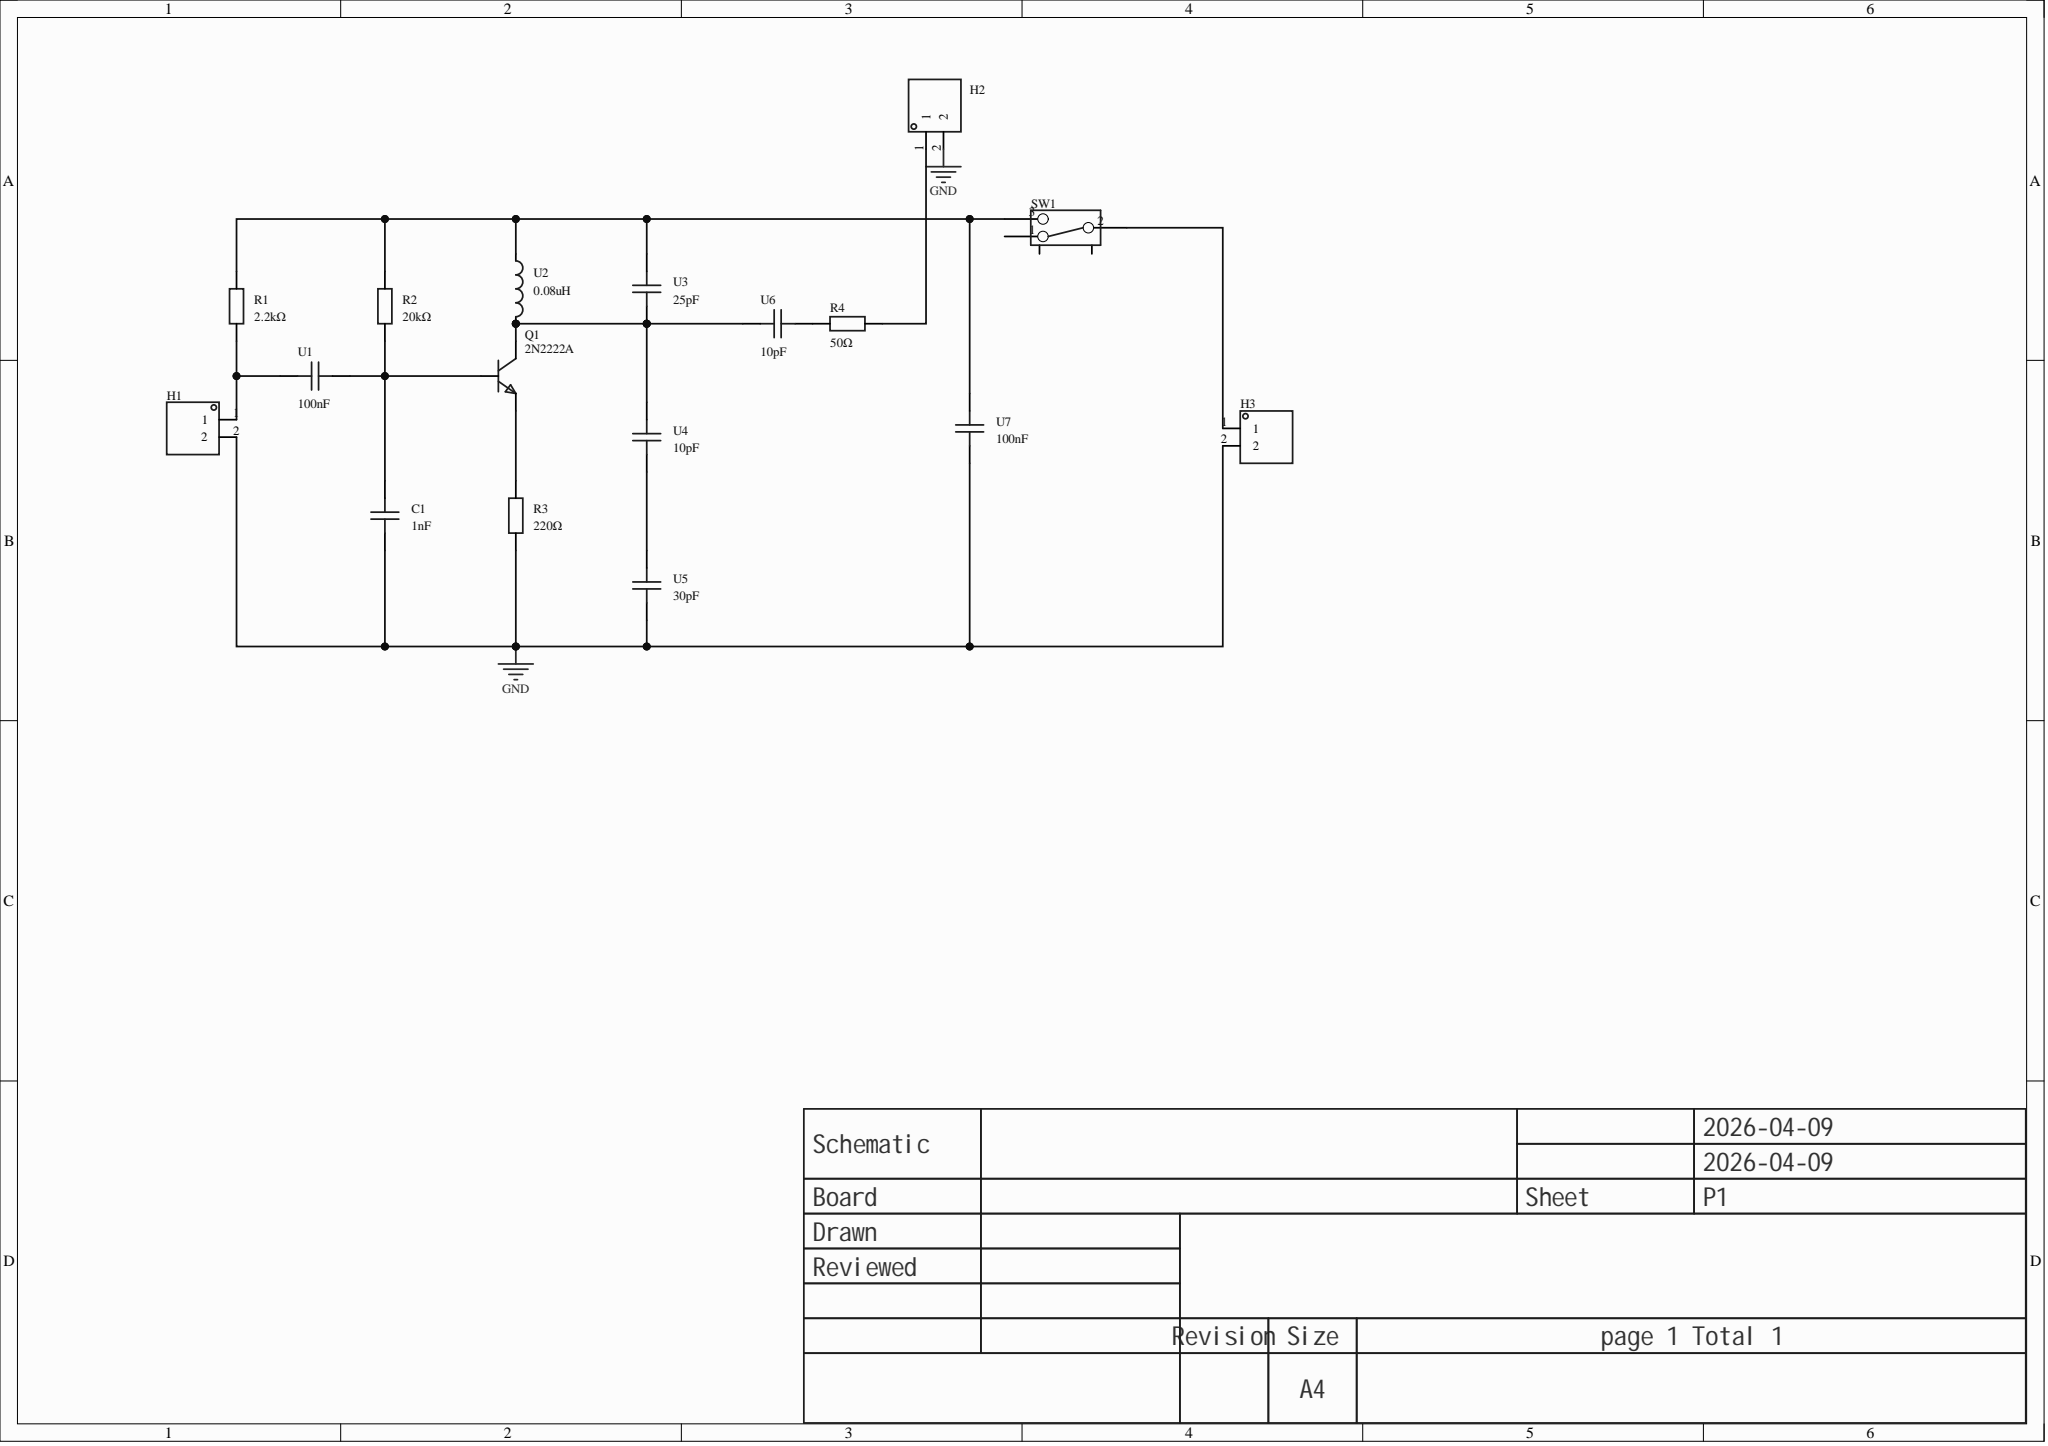Circuit board | Altium Designer | 17 parts | 10 nets
Bill of materials:
Comment,Description,Designator,Footprint,LibRef,Quantity
"1nF","Capacitance: 1nF; Tolerance: ±20%; Working voltage (AC): 400V; 440V; Protection class: X1,Y1;","C1","CAP-TH_L7.0-W4.0-P10.00-D0.6-1","DE1E3RA102MJ4BH01F","1"
"","","H1, H2, H3","HDR-TH_2P-P2.54-V-M-1","HDR-M_2.54_1x2P","3"
"2N2222A","Transistor type: NPN.  Collector current ICM: 800MA  Collector-base breakdown voltage BVCBO: 60V  Collector-emitter breakdown voltage BVCEO: 30V  DC current gain HFE: 100-200","Q1","TO-92-3_L5.1-W4.1-P1.27-L-1","2N2222A_C50229645","1"
"2.2kΩ","","R1","Res_1/8W","Res_AXIAL-1/8W","1"
"20kΩ","","R2","Res_1/8W","Res_AXIAL-1/8W","1"
"220Ω","","R3","Res_1/8W","Res_AXIAL-1/8W","1"
"50Ω","","R4","Res_1/8W","Res_AXIAL-1/8W","1"
"","","SW1","拨动开关_侧","拨动开关_侧","1"
"100nF","","U1, U7","CAP-TH_L5.0-W2.5-P5.00-D1.0","100nF","2"
"0.08uH","Inductance: 1uH; Tolerance: ±10%; Rated current: 4.45A; Saturation current (Isat): 7.7A; Type: color-band inductor; Quality factor: 50@2.52MHz;","U2","IND-TH_BD6.5-W9.2-LS14.0-D0.8","B82144F2102K000","1"
"25pF","","U3","CAP-TH_L5.0-W2.5-P5.00-D1.0","100nF","1"
"10pF","","U4, U6","CAP-TH_L5.0-W2.5-P5.00-D1.0","100nF","2"
"30pF","","U5","CAP-TH_L5.0-W2.5-P5.00-D1.0","100nF","1"
Netlist (Protel format):
[
C1
CAP-TH_L7.0-W4.0-P10.00-D0.6-1
1nF



]
[
H1
HDR-TH_2P-P2.54-V-M-1




]
[
H2
HDR-TH_2P-P2.54-V-M-1




]
[
H3
HDR-TH_2P-P2.54-V-M-1




]
[
Q1
TO-92-3_L5.1-W4.1-P1.27-L-1
2N2222A



]
[
R1
Res_1/8W
2.2kΩ



]
[
R2
Res_1/8W
20kΩ



]
[
R3
Res_1/8W
220Ω



]
[
R4
Res_1/8W
50Ω



]
[
SW1
拨动开关_侧




]
[
U1
CAP-TH_L5.0-W2.5-P5.00-D1.0
100nF



]
[
U2
IND-TH_BD6.5-W9.2-LS14.0-D0.8
0.08uH



]
[
U3
CAP-TH_L5.0-W2.5-P5.00-D1.0
25pF



]
[
U4
CAP-TH_L5.0-W2.5-P5.00-D1.0
10pF



]
[
U5
CAP-TH_L5.0-W2.5-P5.00-D1.0
30pF



]
[
U6
CAP-TH_L5.0-W2.5-P5.00-D1.0
10pF



]
[
U7
CAP-TH_L5.0-W2.5-P5.00-D1.0
100nF



]
(
NetU4_2
U4-2
U5-1
)
(
NetR4_1
R4-1
U6-2
)
(
NetR1_2
R1-2
R2-2
SW1-3
U2-1
U3-1
U7-1
)
(
NetQ1_3
Q1-3
U2-2
U3-2
U4-1
U6-1
)
(
NetQ1_1
Q1-1
R3-2
)
(
NetH3_1
H3-1
SW1-2
)
(
NetH2_1
H2-1
R4-2
)
(
NetH1_1
H1-1
R1-1
U1-2
)
(
NetC1_2
C1-2
Q1-2
R2-1
U1-1
)
(
GND
C1-1
H1-2
H2-2
H3-2
R3-1
U5-2
U7-2
)